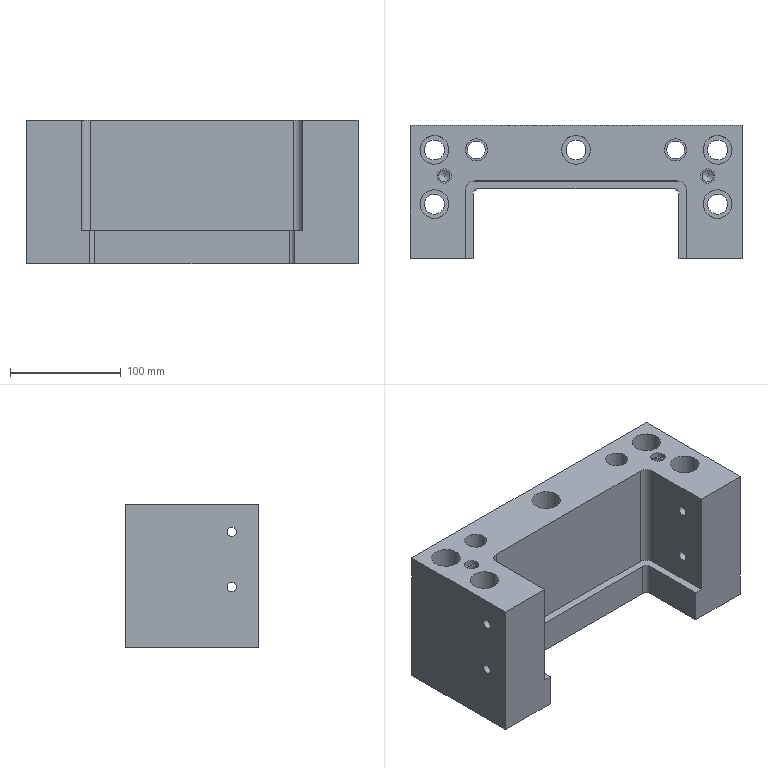Part | NX | features FD 2 | 1 solid | 51 faces | box 300 x 120 x 130 mm | volume 2560198 mm3 | cylinder 26 | plane 23 | cone 2 | commonest cylinder face diameters 18 x5 26 x5 8.5 x4 10 x2 10.3 x2 13 x2
STEP:
#1=CARTESIAN_POINT('',(1053.,-648.5,-33.75));
#2=VERTEX_POINT('',#1);
#3=CARTESIAN_POINT('',(1053.,-648.5,-38.));
#4=DIRECTION('',(-1.,0.,0.));
#5=DIRECTION('',(0.,0.,1.));
#6=AXIS2_PLACEMENT_3D('',#3,#4,#5);
#7=CIRCLE('',#6,4.25);
#8=EDGE_CURVE('',#2,#2,#7,.T.);
#9=ORIENTED_EDGE('',*,*,#8,.T.);
#10=EDGE_LOOP('',(#9));
#11=FACE_BOUND('',#10,.T.);
#12=CARTESIAN_POINT('',(1053.,-648.5,-83.75));
#13=VERTEX_POINT('',#12);
#14=CARTESIAN_POINT('',(1053.,-648.5,-88.));
#15=DIRECTION('',(-1.,0.,0.));
#16=DIRECTION('',(0.,0.,1.));
#17=AXIS2_PLACEMENT_3D('',#14,#15,#16);
#18=CIRCLE('',#17,4.25);
#19=EDGE_CURVE('',#13,#13,#18,.T.);
#20=ORIENTED_EDGE('',*,*,#19,.T.);
#21=EDGE_LOOP('',(#20));
#22=FACE_BOUND('',#21,.T.);
#23=CARTESIAN_POINT('',(1053.,-672.5,-13.));
#24=VERTEX_POINT('',#23);
#25=CARTESIAN_POINT('',(1053.,-672.5,-143.));
#26=VERTEX_POINT('',#25);
#27=CARTESIAN_POINT('',(1053.,-672.5,-3.));
#28=DIRECTION('',(0.,0.,-1.));
#29=VECTOR('',#28,1000.);
#30=LINE('',#27,#29);
#31=EDGE_CURVE('',#24,#26,#30,.T.);
#32=ORIENTED_EDGE('',*,*,#31,.T.);
#33=CARTESIAN_POINT('',(1053.,-552.5,-143.));
#34=VERTEX_POINT('',#33);
#35=CARTESIAN_POINT('',(1053.,-639.99,-143.));
#36=DIRECTION('',(0.,-1.,0.));
#37=VECTOR('',#36,1000.);
#38=LINE('',#35,#37);
#39=EDGE_CURVE('',#34,#26,#38,.T.);
#40=ORIENTED_EDGE('',*,*,#39,.F.);
#41=CARTESIAN_POINT('',(1053.,-552.5,-13.));
#42=VERTEX_POINT('',#41);
#43=CARTESIAN_POINT('',(1053.,-552.5,-3.));
#44=DIRECTION('',(0.,0.,-1.));
#45=VECTOR('',#44,1000.);
#46=LINE('',#43,#45);
#47=EDGE_CURVE('',#42,#34,#46,.T.);
#48=ORIENTED_EDGE('',*,*,#47,.F.);
#49=CARTESIAN_POINT('',(1053.,-667.5,-13.));
#50=DIRECTION('',(0.,-1.,0.));
#51=VECTOR('',#50,1000.);
#52=LINE('',#49,#51);
#53=EDGE_CURVE('',#42,#24,#52,.T.);
#54=ORIENTED_EDGE('',*,*,#53,.T.);
#55=EDGE_LOOP('',(#32,#40,#48,#54));
#56=FACE_BOUND('',#55,.T.);
#57=CARTESIAN_POINT('',(1053.,-667.5,202.));
#58=DIRECTION('',(-1.,0.,0.));
#59=DIRECTION('',(0.,0.,-1.));
#60=AXIS2_PLACEMENT_3D('',#57,#58,#59);
#61=PLANE('',#60);
#62=ADVANCED_FACE('',(#11,#22,#56),#61,.F.);
#63=CARTESIAN_POINT('',(803.,-648.5,-42.25));
#64=VERTEX_POINT('',#63);
#65=CARTESIAN_POINT('',(803.,-648.5,-38.));
#66=DIRECTION('',(1.,0.,0.));
#67=DIRECTION('',(0.,0.,-1.));
#68=AXIS2_PLACEMENT_3D('',#65,#66,#67);
#69=CIRCLE('',#68,4.25);
#70=EDGE_CURVE('',#64,#64,#69,.T.);
#71=ORIENTED_EDGE('',*,*,#70,.F.);
#72=EDGE_LOOP('',(#71));
#73=FACE_BOUND('',#72,.T.);
#74=CARTESIAN_POINT('',(803.,-648.5,-92.25));
#75=VERTEX_POINT('',#74);
#76=CARTESIAN_POINT('',(803.,-648.5,-88.));
#77=DIRECTION('',(1.,0.,0.));
#78=DIRECTION('',(0.,0.,-1.));
#79=AXIS2_PLACEMENT_3D('',#76,#77,#78);
#80=CIRCLE('',#79,4.25);
#81=EDGE_CURVE('',#75,#75,#80,.T.);
#82=ORIENTED_EDGE('',*,*,#81,.F.);
#83=EDGE_LOOP('',(#82));
#84=FACE_BOUND('',#83,.T.);
#85=CARTESIAN_POINT('',(803.,-672.5,-113.));
#86=VERTEX_POINT('',#85);
#87=CARTESIAN_POINT('',(803.,-610.5,-113.));
#88=VERTEX_POINT('',#87);
#89=CARTESIAN_POINT('',(803.,-674.98,-113.));
#90=DIRECTION('',(0.,1.,0.));
#91=VECTOR('',#90,1000.);
#92=LINE('',#89,#91);
#93=EDGE_CURVE('',#86,#88,#92,.T.);
#94=ORIENTED_EDGE('',*,*,#93,.T.);
#95=CARTESIAN_POINT('',(803.,-610.5,-13.));
#96=VERTEX_POINT('',#95);
#97=CARTESIAN_POINT('',(803.,-610.5,-113.));
#98=DIRECTION('',(0.,0.,-1.));
#99=VECTOR('',#98,1000.);
#100=LINE('',#97,#99);
#101=EDGE_CURVE('',#96,#88,#100,.T.);
#102=ORIENTED_EDGE('',*,*,#101,.F.);
#103=CARTESIAN_POINT('',(803.,-672.5,-13.));
#104=VERTEX_POINT('',#103);
#105=CARTESIAN_POINT('',(803.,-674.98,-13.));
#106=DIRECTION('',(0.,1.,0.));
#107=VECTOR('',#106,1000.);
#108=LINE('',#105,#107);
#109=EDGE_CURVE('',#104,#96,#108,.T.);
#110=ORIENTED_EDGE('',*,*,#109,.F.);
#111=CARTESIAN_POINT('',(803.,-672.5,-3.));
#112=DIRECTION('',(0.,0.,1.));
#113=VECTOR('',#112,1000.);
#114=LINE('',#111,#113);
#115=EDGE_CURVE('',#86,#104,#114,.T.);
#116=ORIENTED_EDGE('',*,*,#115,.F.);
#117=EDGE_LOOP('',(#94,#102,#110,#116));
#118=FACE_BOUND('',#117,.T.);
#119=CARTESIAN_POINT('',(803.,-674.98,-113.));
#120=DIRECTION('',(-1.,0.,0.));
#121=DIRECTION('',(0.,0.,1.));
#122=AXIS2_PLACEMENT_3D('',#119,#120,#121);
#123=PLANE('',#122);
#124=ADVANCED_FACE('',(#73,#84,#118),#123,.F.);
#125=CARTESIAN_POINT('',(811.,-602.5,-113.));
#126=VERTEX_POINT('',#125);
#127=CARTESIAN_POINT('',(811.,-610.5,-113.));
#128=DIRECTION('',(0.,0.,-1.));
#129=DIRECTION('',(-1.,0.,0.));
#130=AXIS2_PLACEMENT_3D('',#127,#128,#129);
#131=CIRCLE('',#130,8.);
#132=EDGE_CURVE('',#88,#126,#131,.T.);
#133=ORIENTED_EDGE('',*,*,#132,.T.);
#134=CARTESIAN_POINT('',(811.,-602.5,-13.));
#135=VERTEX_POINT('',#134);
#136=CARTESIAN_POINT('',(811.,-602.5,-13.));
#137=DIRECTION('',(0.,0.,1.));
#138=VECTOR('',#137,1000.);
#139=LINE('',#136,#138);
#140=EDGE_CURVE('',#126,#135,#139,.T.);
#141=ORIENTED_EDGE('',*,*,#140,.T.);
#142=CARTESIAN_POINT('',(811.,-610.5,-13.));
#143=DIRECTION('',(0.,0.,1.));
#144=DIRECTION('',(-1.,0.,0.));
#145=AXIS2_PLACEMENT_3D('',#142,#143,#144);
#146=CIRCLE('',#145,8.);
#147=EDGE_CURVE('',#135,#96,#146,.T.);
#148=ORIENTED_EDGE('',*,*,#147,.T.);
#149=ORIENTED_EDGE('',*,*,#101,.T.);
#150=EDGE_LOOP('',(#133,#141,#148,#149));
#151=FACE_BOUND('',#150,.T.);
#152=CARTESIAN_POINT('',(811.,-610.5,-113.));
#153=DIRECTION('',(0.,0.,1.));
#154=DIRECTION('',(-1.,0.,0.));
#155=AXIS2_PLACEMENT_3D('',#152,#153,#154);
#156=CYLINDRICAL_SURFACE('',#155,8.);
#157=ADVANCED_FACE('',(#151),#156,.F.);
#158=CARTESIAN_POINT('',(995.,-602.5,-113.));
#159=VERTEX_POINT('',#158);
#160=CARTESIAN_POINT('',(832.96,-602.5,-113.));
#161=DIRECTION('',(-1.,0.,0.));
#162=VECTOR('',#161,1000.);
#163=LINE('',#160,#162);
#164=EDGE_CURVE('',#159,#126,#163,.T.);
#165=ORIENTED_EDGE('',*,*,#164,.F.);
#166=CARTESIAN_POINT('',(995.,-602.5,-13.));
#167=VERTEX_POINT('',#166);
#168=CARTESIAN_POINT('',(995.,-602.5,-113.));
#169=DIRECTION('',(0.,0.,-1.));
#170=VECTOR('',#169,1000.);
#171=LINE('',#168,#170);
#172=EDGE_CURVE('',#167,#159,#171,.T.);
#173=ORIENTED_EDGE('',*,*,#172,.F.);
#174=CARTESIAN_POINT('',(832.96,-602.5,-13.));
#175=DIRECTION('',(1.,0.,0.));
#176=VECTOR('',#175,1000.);
#177=LINE('',#174,#176);
#178=EDGE_CURVE('',#135,#167,#177,.T.);
#179=ORIENTED_EDGE('',*,*,#178,.F.);
#180=ORIENTED_EDGE('',*,*,#140,.F.);
#181=EDGE_LOOP('',(#165,#173,#179,#180));
#182=FACE_BOUND('',#181,.T.);
#183=CARTESIAN_POINT('',(832.96,-602.5,-113.));
#184=DIRECTION('',(0.,1.,0.));
#185=DIRECTION('',(0.,0.,-1.));
#186=AXIS2_PLACEMENT_3D('',#183,#184,#185);
#187=PLANE('',#186);
#188=ADVANCED_FACE('',(#182),#187,.F.);
#189=CARTESIAN_POINT('',(1003.,-610.5,-113.));
#190=VERTEX_POINT('',#189);
#191=CARTESIAN_POINT('',(995.,-610.5,-113.));
#192=DIRECTION('',(0.,0.,1.));
#193=DIRECTION('',(-1.,0.,0.));
#194=AXIS2_PLACEMENT_3D('',#191,#192,#193);
#195=CIRCLE('',#194,8.);
#196=EDGE_CURVE('',#190,#159,#195,.T.);
#197=ORIENTED_EDGE('',*,*,#196,.F.);
#198=CARTESIAN_POINT('',(1003.,-610.5,-13.));
#199=VERTEX_POINT('',#198);
#200=CARTESIAN_POINT('',(1003.,-610.5,-113.));
#201=DIRECTION('',(0.,0.,1.));
#202=VECTOR('',#201,1000.);
#203=LINE('',#200,#202);
#204=EDGE_CURVE('',#190,#199,#203,.T.);
#205=ORIENTED_EDGE('',*,*,#204,.T.);
#206=CARTESIAN_POINT('',(995.,-610.5,-13.));
#207=DIRECTION('',(0.,0.,1.));
#208=DIRECTION('',(-1.,0.,0.));
#209=AXIS2_PLACEMENT_3D('',#206,#207,#208);
#210=CIRCLE('',#209,8.);
#211=EDGE_CURVE('',#199,#167,#210,.T.);
#212=ORIENTED_EDGE('',*,*,#211,.T.);
#213=ORIENTED_EDGE('',*,*,#172,.T.);
#214=EDGE_LOOP('',(#197,#205,#212,#213));
#215=FACE_BOUND('',#214,.T.);
#216=CARTESIAN_POINT('',(995.,-610.5,-113.));
#217=DIRECTION('',(0.,0.,1.));
#218=DIRECTION('',(-1.,0.,0.));
#219=AXIS2_PLACEMENT_3D('',#216,#217,#218);
#220=CYLINDRICAL_SURFACE('',#219,8.);
#221=ADVANCED_FACE('',(#215),#220,.F.);
#222=CARTESIAN_POINT('',(1003.,-648.5,-33.75));
#223=VERTEX_POINT('',#222);
#224=CARTESIAN_POINT('',(1003.,-648.5,-38.));
#225=DIRECTION('',(-1.,0.,0.));
#226=DIRECTION('',(0.,0.,1.));
#227=AXIS2_PLACEMENT_3D('',#224,#225,#226);
#228=CIRCLE('',#227,4.25);
#229=EDGE_CURVE('',#223,#223,#228,.T.);
#230=ORIENTED_EDGE('',*,*,#229,.F.);
#231=EDGE_LOOP('',(#230));
#232=FACE_BOUND('',#231,.T.);
#233=CARTESIAN_POINT('',(1003.,-648.5,-83.75));
#234=VERTEX_POINT('',#233);
#235=CARTESIAN_POINT('',(1003.,-648.5,-88.));
#236=DIRECTION('',(-1.,0.,0.));
#237=DIRECTION('',(0.,0.,1.));
#238=AXIS2_PLACEMENT_3D('',#235,#236,#237);
#239=CIRCLE('',#238,4.25);
#240=EDGE_CURVE('',#234,#234,#239,.T.);
#241=ORIENTED_EDGE('',*,*,#240,.F.);
#242=EDGE_LOOP('',(#241));
#243=FACE_BOUND('',#242,.T.);
#244=CARTESIAN_POINT('',(1003.,-672.5,-113.));
#245=VERTEX_POINT('',#244);
#246=CARTESIAN_POINT('',(1003.,-612.48,-113.));
#247=DIRECTION('',(0.,1.,0.));
#248=VECTOR('',#247,1000.);
#249=LINE('',#246,#248);
#250=EDGE_CURVE('',#245,#190,#249,.T.);
#251=ORIENTED_EDGE('',*,*,#250,.F.);
#252=CARTESIAN_POINT('',(1003.,-672.5,-13.));
#253=VERTEX_POINT('',#252);
#254=CARTESIAN_POINT('',(1003.,-672.5,-3.));
#255=DIRECTION('',(0.,0.,-1.));
#256=VECTOR('',#255,1000.);
#257=LINE('',#254,#256);
#258=EDGE_CURVE('',#253,#245,#257,.T.);
#259=ORIENTED_EDGE('',*,*,#258,.F.);
#260=CARTESIAN_POINT('',(1003.,-612.48,-13.));
#261=DIRECTION('',(0.,-1.,0.));
#262=VECTOR('',#261,1000.);
#263=LINE('',#260,#262);
#264=EDGE_CURVE('',#199,#253,#263,.T.);
#265=ORIENTED_EDGE('',*,*,#264,.F.);
#266=ORIENTED_EDGE('',*,*,#204,.F.);
#267=EDGE_LOOP('',(#251,#259,#265,#266));
#268=FACE_BOUND('',#267,.T.);
#269=CARTESIAN_POINT('',(1003.,-612.48,-113.));
#270=DIRECTION('',(1.,0.,0.));
#271=DIRECTION('',(0.,0.,-1.));
#272=AXIS2_PLACEMENT_3D('',#269,#270,#271);
#273=PLANE('',#272);
#274=ADVANCED_FACE('',(#232,#243,#268),#273,.F.);
#275=ORIENTED_EDGE('',*,*,#258,.T.);
#276=CARTESIAN_POINT('',(996.,-672.5,-113.));
#277=VERTEX_POINT('',#276);
#278=CARTESIAN_POINT('',(1007.98,-672.5,-113.));
#279=DIRECTION('',(1.,0.,0.));
#280=VECTOR('',#279,1000.);
#281=LINE('',#278,#280);
#282=EDGE_CURVE('',#277,#245,#281,.T.);
#283=ORIENTED_EDGE('',*,*,#282,.F.);
#284=CARTESIAN_POINT('',(996.,-672.5,-143.));
#285=VERTEX_POINT('',#284);
#286=CARTESIAN_POINT('',(996.,-672.5,-113.));
#287=DIRECTION('',(0.,0.,-1.));
#288=VECTOR('',#287,1000.);
#289=LINE('',#286,#288);
#290=EDGE_CURVE('',#277,#285,#289,.T.);
#291=ORIENTED_EDGE('',*,*,#290,.T.);
#292=CARTESIAN_POINT('',(1007.98,-672.5,-143.));
#293=DIRECTION('',(-1.,0.,0.));
#294=VECTOR('',#293,1000.);
#295=LINE('',#292,#294);
#296=EDGE_CURVE('',#26,#285,#295,.T.);
#297=ORIENTED_EDGE('',*,*,#296,.F.);
#298=ORIENTED_EDGE('',*,*,#31,.F.);
#299=CARTESIAN_POINT('',(1007.98,-672.5,-13.));
#300=DIRECTION('',(1.,0.,0.));
#301=VECTOR('',#300,1000.);
#302=LINE('',#299,#301);
#303=EDGE_CURVE('',#253,#24,#302,.T.);
#304=ORIENTED_EDGE('',*,*,#303,.F.);
#305=EDGE_LOOP('',(#275,#283,#291,#297,#298,#304));
#306=FACE_BOUND('',#305,.T.);
#307=CARTESIAN_POINT('',(1007.98,-672.5,-3.));
#308=DIRECTION('',(0.,-1.,0.));
#309=DIRECTION('',(0.,0.,1.));
#310=AXIS2_PLACEMENT_3D('',#307,#308,#309);
#311=PLANE('',#310);
#312=ADVANCED_FACE('',(#306),#311,.T.);
#313=CARTESIAN_POINT('',(753.,-672.5,-13.));
#314=VERTEX_POINT('',#313);
#315=CARTESIAN_POINT('',(753.,-672.5,-143.));
#316=VERTEX_POINT('',#315);
#317=CARTESIAN_POINT('',(753.,-672.5,202.));
#318=DIRECTION('',(0.,0.,-1.));
#319=VECTOR('',#318,1000.);
#320=LINE('',#317,#319);
#321=EDGE_CURVE('',#314,#316,#320,.T.);
#322=ORIENTED_EDGE('',*,*,#321,.T.);
#323=CARTESIAN_POINT('',(810.,-672.5,-143.));
#324=VERTEX_POINT('',#323);
#325=CARTESIAN_POINT('',(797.98,-672.5,-143.));
#326=DIRECTION('',(-1.,0.,0.));
#327=VECTOR('',#326,1000.);
#328=LINE('',#325,#327);
#329=EDGE_CURVE('',#324,#316,#328,.T.);
#330=ORIENTED_EDGE('',*,*,#329,.F.);
#331=CARTESIAN_POINT('',(810.,-672.5,-113.));
#332=VERTEX_POINT('',#331);
#333=CARTESIAN_POINT('',(810.,-672.5,-3.));
#334=DIRECTION('',(0.,0.,1.));
#335=VECTOR('',#334,1000.);
#336=LINE('',#333,#335);
#337=EDGE_CURVE('',#324,#332,#336,.T.);
#338=ORIENTED_EDGE('',*,*,#337,.T.);
#339=CARTESIAN_POINT('',(797.98,-672.5,-113.));
#340=DIRECTION('',(1.,0.,0.));
#341=VECTOR('',#340,1000.);
#342=LINE('',#339,#341);
#343=EDGE_CURVE('',#86,#332,#342,.T.);
#344=ORIENTED_EDGE('',*,*,#343,.F.);
#345=ORIENTED_EDGE('',*,*,#115,.T.);
#346=CARTESIAN_POINT('',(797.98,-672.5,-13.));
#347=DIRECTION('',(-1.,0.,0.));
#348=VECTOR('',#347,1000.);
#349=LINE('',#346,#348);
#350=EDGE_CURVE('',#104,#314,#349,.T.);
#351=ORIENTED_EDGE('',*,*,#350,.T.);
#352=EDGE_LOOP('',(#322,#330,#338,#344,#345,#351));
#353=FACE_BOUND('',#352,.T.);
#354=CARTESIAN_POINT('',(797.98,-672.5,-3.));
#355=DIRECTION('',(0.,1.,0.));
#356=DIRECTION('',(0.,0.,1.));
#357=AXIS2_PLACEMENT_3D('',#354,#355,#356);
#358=PLANE('',#357);
#359=ADVANCED_FACE('',(#353),#358,.F.);
#360=CARTESIAN_POINT('',(753.,-648.5,-42.25));
#361=VERTEX_POINT('',#360);
#362=CARTESIAN_POINT('',(753.,-648.5,-38.));
#363=DIRECTION('',(1.,0.,0.));
#364=DIRECTION('',(0.,0.,-1.));
#365=AXIS2_PLACEMENT_3D('',#362,#363,#364);
#366=CIRCLE('',#365,4.25);
#367=EDGE_CURVE('',#361,#361,#366,.T.);
#368=ORIENTED_EDGE('',*,*,#367,.T.);
#369=EDGE_LOOP('',(#368));
#370=FACE_BOUND('',#369,.T.);
#371=CARTESIAN_POINT('',(753.,-648.5,-92.25));
#372=VERTEX_POINT('',#371);
#373=CARTESIAN_POINT('',(753.,-648.5,-88.));
#374=DIRECTION('',(1.,0.,0.));
#375=DIRECTION('',(0.,0.,-1.));
#376=AXIS2_PLACEMENT_3D('',#373,#374,#375);
#377=CIRCLE('',#376,4.25);
#378=EDGE_CURVE('',#372,#372,#377,.T.);
#379=ORIENTED_EDGE('',*,*,#378,.T.);
#380=EDGE_LOOP('',(#379));
#381=FACE_BOUND('',#380,.T.);
#382=CARTESIAN_POINT('',(753.,-552.5,-13.));
#383=VERTEX_POINT('',#382);
#384=CARTESIAN_POINT('',(753.,-552.5,-143.));
#385=VERTEX_POINT('',#384);
#386=CARTESIAN_POINT('',(753.,-552.5,202.));
#387=DIRECTION('',(0.,0.,-1.));
#388=VECTOR('',#387,1000.);
#389=LINE('',#386,#388);
#390=EDGE_CURVE('',#383,#385,#389,.T.);
#391=ORIENTED_EDGE('',*,*,#390,.T.);
#392=CARTESIAN_POINT('',(753.,-639.99,-143.));
#393=DIRECTION('',(0.,1.,0.));
#394=VECTOR('',#393,1000.);
#395=LINE('',#392,#394);
#396=EDGE_CURVE('',#316,#385,#395,.T.);
#397=ORIENTED_EDGE('',*,*,#396,.F.);
#398=ORIENTED_EDGE('',*,*,#321,.F.);
#399=CARTESIAN_POINT('',(753.,-667.5,-13.));
#400=DIRECTION('',(0.,1.,0.));
#401=VECTOR('',#400,1000.);
#402=LINE('',#399,#401);
#403=EDGE_CURVE('',#314,#383,#402,.T.);
#404=ORIENTED_EDGE('',*,*,#403,.T.);
#405=EDGE_LOOP('',(#391,#397,#398,#404));
#406=FACE_BOUND('',#405,.T.);
#407=CARTESIAN_POINT('',(753.,-622.5,202.));
#408=DIRECTION('',(1.,0.,0.));
#409=DIRECTION('',(0.,0.,1.));
#410=AXIS2_PLACEMENT_3D('',#407,#408,#409);
#411=PLANE('',#410);
#412=ADVANCED_FACE('',(#370,#381,#406),#411,.F.);
#413=ORIENTED_EDGE('',*,*,#47,.T.);
#414=CARTESIAN_POINT('',(827.98,-552.5,-143.));
#415=DIRECTION('',(1.,0.,0.));
#416=VECTOR('',#415,1000.);
#417=LINE('',#414,#416);
#418=EDGE_CURVE('',#385,#34,#417,.T.);
#419=ORIENTED_EDGE('',*,*,#418,.F.);
#420=ORIENTED_EDGE('',*,*,#390,.F.);
#421=CARTESIAN_POINT('',(827.98,-552.5,-13.));
#422=DIRECTION('',(1.,0.,0.));
#423=VECTOR('',#422,1000.);
#424=LINE('',#421,#423);
#425=EDGE_CURVE('',#383,#42,#424,.T.);
#426=ORIENTED_EDGE('',*,*,#425,.T.);
#427=EDGE_LOOP('',(#413,#419,#420,#426));
#428=FACE_BOUND('',#427,.T.);
#429=CARTESIAN_POINT('',(827.98,-552.5,-3.));
#430=DIRECTION('',(0.,-1.,0.));
#431=DIRECTION('',(0.,0.,1.));
#432=AXIS2_PLACEMENT_3D('',#429,#430,#431);
#433=PLANE('',#432);
#434=ADVANCED_FACE('',(#428),#433,.F.);
#435=CARTESIAN_POINT('',(985.,-574.5,-67.));
#436=VERTEX_POINT('',#435);
#437=CARTESIAN_POINT('',(993.,-574.5,-67.));
#438=DIRECTION('',(0.,0.,-1.));
#439=DIRECTION('',(-1.,0.,0.));
#440=AXIS2_PLACEMENT_3D('',#437,#438,#439);
#441=CIRCLE('',#440,8.001);
#442=EDGE_CURVE('',#436,#436,#441,.T.);
#443=ORIENTED_EDGE('',*,*,#442,.F.);
#444=EDGE_LOOP('',(#443));
#445=FACE_BOUND('',#444,.T.);
#446=CARTESIAN_POINT('',(1001.,-574.5,-143.));
#447=VERTEX_POINT('',#446);
#448=CARTESIAN_POINT('',(993.,-574.5,-143.));
#449=DIRECTION('',(0.,0.,1.));
#450=DIRECTION('',(1.,0.,0.));
#451=AXIS2_PLACEMENT_3D('',#448,#449,#450);
#452=CIRCLE('',#451,8.001);
#453=EDGE_CURVE('',#447,#447,#452,.T.);
#454=ORIENTED_EDGE('',*,*,#453,.F.);
#455=EDGE_LOOP('',(#454));
#456=FACE_BOUND('',#455,.T.);
#457=CARTESIAN_POINT('',(993.,-574.5,-11.));
#458=DIRECTION('',(0.,0.,-1.));
#459=DIRECTION('',(1.,0.,0.));
#460=AXIS2_PLACEMENT_3D('',#457,#458,#459);
#461=CYLINDRICAL_SURFACE('',#460,8.001);
#462=ADVANCED_FACE('',(#445,#456),#461,.F.);
#463=CARTESIAN_POINT('',(1022.,-623.5,-103.));
#464=VERTEX_POINT('',#463);
#465=CARTESIAN_POINT('',(1031.,-623.5,-103.));
#466=DIRECTION('',(0.,0.,-1.));
#467=DIRECTION('',(-1.,0.,0.));
#468=AXIS2_PLACEMENT_3D('',#465,#466,#467);
#469=CIRCLE('',#468,9.);
#470=EDGE_CURVE('',#464,#464,#469,.T.);
#471=ORIENTED_EDGE('',*,*,#470,.F.);
#472=EDGE_LOOP('',(#471));
#473=FACE_BOUND('',#472,.T.);
#474=CARTESIAN_POINT('',(1040.,-623.5,-143.));
#475=VERTEX_POINT('',#474);
#476=CARTESIAN_POINT('',(1031.,-623.5,-143.));
#477=DIRECTION('',(0.,0.,1.));
#478=DIRECTION('',(1.,0.,0.));
#479=AXIS2_PLACEMENT_3D('',#476,#477,#478);
#480=CIRCLE('',#479,9.);
#481=EDGE_CURVE('',#475,#475,#480,.T.);
#482=ORIENTED_EDGE('',*,*,#481,.F.);
#483=EDGE_LOOP('',(#482));
#484=FACE_BOUND('',#483,.T.);
#485=CARTESIAN_POINT('',(1031.,-623.5,-11.));
#486=DIRECTION('',(0.,0.,-1.));
#487=DIRECTION('',(-1.,0.,0.));
#488=AXIS2_PLACEMENT_3D('',#485,#486,#487);
#489=CYLINDRICAL_SURFACE('',#488,9.);
#490=ADVANCED_FACE('',(#473,#484),#489,.F.);
#491=CARTESIAN_POINT('',(766.,-574.5,-103.));
#492=VERTEX_POINT('',#491);
#493=CARTESIAN_POINT('',(775.,-574.5,-103.));
#494=DIRECTION('',(0.,0.,-1.));
#495=DIRECTION('',(-1.,0.,0.));
#496=AXIS2_PLACEMENT_3D('',#493,#494,#495);
#497=CIRCLE('',#496,9.);
#498=EDGE_CURVE('',#492,#492,#497,.T.);
#499=ORIENTED_EDGE('',*,*,#498,.F.);
#500=EDGE_LOOP('',(#499));
#501=FACE_BOUND('',#500,.T.);
#502=CARTESIAN_POINT('',(784.,-574.5,-143.));
#503=VERTEX_POINT('',#502);
#504=CARTESIAN_POINT('',(775.,-574.5,-143.));
#505=DIRECTION('',(0.,0.,1.));
#506=DIRECTION('',(1.,0.,0.));
#507=AXIS2_PLACEMENT_3D('',#504,#505,#506);
#508=CIRCLE('',#507,9.);
#509=EDGE_CURVE('',#503,#503,#508,.T.);
#510=ORIENTED_EDGE('',*,*,#509,.F.);
#511=EDGE_LOOP('',(#510));
#512=FACE_BOUND('',#511,.T.);
#513=CARTESIAN_POINT('',(775.,-574.5,-11.));
#514=DIRECTION('',(0.,0.,-1.));
#515=DIRECTION('',(-1.,0.,0.));
#516=AXIS2_PLACEMENT_3D('',#513,#514,#515);
#517=CYLINDRICAL_SURFACE('',#516,9.);
#518=ADVANCED_FACE('',(#501,#512),#517,.F.);
#519=CARTESIAN_POINT('',(894.,-574.5,-103.));
#520=VERTEX_POINT('',#519);
#521=CARTESIAN_POINT('',(903.,-574.5,-103.));
#522=DIRECTION('',(0.,0.,-1.));
#523=DIRECTION('',(-1.,0.,0.));
#524=AXIS2_PLACEMENT_3D('',#521,#522,#523);
#525=CIRCLE('',#524,9.);
#526=EDGE_CURVE('',#520,#520,#525,.T.);
#527=ORIENTED_EDGE('',*,*,#526,.F.);
#528=EDGE_LOOP('',(#527));
#529=FACE_BOUND('',#528,.T.);
#530=CARTESIAN_POINT('',(912.,-574.5,-143.));
#531=VERTEX_POINT('',#530);
#532=CARTESIAN_POINT('',(903.,-574.5,-143.));
#533=DIRECTION('',(0.,0.,1.));
#534=DIRECTION('',(1.,0.,0.));
#535=AXIS2_PLACEMENT_3D('',#532,#533,#534);
#536=CIRCLE('',#535,9.);
#537=EDGE_CURVE('',#531,#531,#536,.T.);
#538=ORIENTED_EDGE('',*,*,#537,.F.);
#539=EDGE_LOOP('',(#538));
#540=FACE_BOUND('',#539,.T.);
#541=CARTESIAN_POINT('',(903.,-574.5,-11.));
#542=DIRECTION('',(0.,0.,-1.));
#543=DIRECTION('',(-1.,0.,0.));
#544=AXIS2_PLACEMENT_3D('',#541,#542,#543);
#545=CYLINDRICAL_SURFACE('',#544,9.);
#546=ADVANCED_FACE('',(#529,#540),#545,.F.);
#547=CARTESIAN_POINT('',(1022.,-574.5,-103.));
#548=VERTEX_POINT('',#547);
#549=CARTESIAN_POINT('',(1031.,-574.5,-103.));
#550=DIRECTION('',(0.,0.,-1.));
#551=DIRECTION('',(-1.,0.,0.));
#552=AXIS2_PLACEMENT_3D('',#549,#550,#551);
#553=CIRCLE('',#552,9.);
#554=EDGE_CURVE('',#548,#548,#553,.T.);
#555=ORIENTED_EDGE('',*,*,#554,.F.);
#556=EDGE_LOOP('',(#555));
#557=FACE_BOUND('',#556,.T.);
#558=CARTESIAN_POINT('',(1040.,-574.5,-143.));
#559=VERTEX_POINT('',#558);
#560=CARTESIAN_POINT('',(1031.,-574.5,-143.));
#561=DIRECTION('',(0.,0.,1.));
#562=DIRECTION('',(1.,0.,0.));
#563=AXIS2_PLACEMENT_3D('',#560,#561,#562);
#564=CIRCLE('',#563,9.);
#565=EDGE_CURVE('',#559,#559,#564,.T.);
#566=ORIENTED_EDGE('',*,*,#565,.F.);
#567=EDGE_LOOP('',(#566));
#568=FACE_BOUND('',#567,.T.);
#569=CARTESIAN_POINT('',(1031.,-574.5,-11.));
#570=DIRECTION('',(0.,0.,-1.));
#571=DIRECTION('',(-1.,0.,0.));
#572=AXIS2_PLACEMENT_3D('',#569,#570,#571);
#573=CYLINDRICAL_SURFACE('',#572,9.);
#574=ADVANCED_FACE('',(#557,#568),#573,.F.);
#575=CARTESIAN_POINT('',(805.,-574.5,-67.));
#576=VERTEX_POINT('',#575);
#577=CARTESIAN_POINT('',(813.,-574.5,-67.));
#578=DIRECTION('',(0.,0.,-1.));
#579=DIRECTION('',(-1.,0.,0.));
#580=AXIS2_PLACEMENT_3D('',#577,#578,#579);
#581=CIRCLE('',#580,8.001);
#582=EDGE_CURVE('',#576,#576,#581,.T.);
#583=ORIENTED_EDGE('',*,*,#582,.F.);
#584=EDGE_LOOP('',(#583));
#585=FACE_BOUND('',#584,.T.);
#586=CARTESIAN_POINT('',(821.,-574.5,-143.));
#587=VERTEX_POINT('',#586);
#588=CARTESIAN_POINT('',(813.,-574.5,-143.));
#589=DIRECTION('',(0.,0.,1.));
#590=DIRECTION('',(1.,0.,0.));
#591=AXIS2_PLACEMENT_3D('',#588,#589,#590);
#592=CIRCLE('',#591,8.001);
#593=EDGE_CURVE('',#587,#587,#592,.T.);
#594=ORIENTED_EDGE('',*,*,#593,.F.);
#595=EDGE_LOOP('',(#594));
#596=FACE_BOUND('',#595,.T.);
#597=CARTESIAN_POINT('',(813.,-574.5,-11.));
#598=DIRECTION('',(0.,0.,-1.));
#599=DIRECTION('',(-1.,0.,0.));
#600=AXIS2_PLACEMENT_3D('',#597,#598,#599);
#601=CYLINDRICAL_SURFACE('',#600,8.001);
#602=ADVANCED_FACE('',(#585,#596),#601,.F.);
#603=CARTESIAN_POINT('',(766.,-623.5,-103.));
#604=VERTEX_POINT('',#603);
#605=CARTESIAN_POINT('',(775.,-623.5,-103.));
#606=DIRECTION('',(0.,0.,-1.));
#607=DIRECTION('',(-1.,0.,0.));
#608=AXIS2_PLACEMENT_3D('',#605,#606,#607);
#609=CIRCLE('',#608,9.);
#610=EDGE_CURVE('',#604,#604,#609,.T.);
#611=ORIENTED_EDGE('',*,*,#610,.F.);
#612=EDGE_LOOP('',(#611));
#613=FACE_BOUND('',#612,.T.);
#614=CARTESIAN_POINT('',(784.,-623.5,-143.));
#615=VERTEX_POINT('',#614);
#616=CARTESIAN_POINT('',(775.,-623.5,-143.));
#617=DIRECTION('',(0.,0.,1.));
#618=DIRECTION('',(1.,0.,0.));
#619=AXIS2_PLACEMENT_3D('',#616,#617,#618);
#620=CIRCLE('',#619,9.);
#621=EDGE_CURVE('',#615,#615,#620,.T.);
#622=ORIENTED_EDGE('',*,*,#621,.F.);
#623=EDGE_LOOP('',(#622));
#624=FACE_BOUND('',#623,.T.);
#625=CARTESIAN_POINT('',(775.,-623.5,-11.));
#626=DIRECTION('',(0.,0.,-1.));
#627=DIRECTION('',(-1.,0.,0.));
#628=AXIS2_PLACEMENT_3D('',#625,#626,#627);
#629=CYLINDRICAL_SURFACE('',#628,9.);
#630=ADVANCED_FACE('',(#613,#624),#629,.F.);
#631=CARTESIAN_POINT('',(1028.595,-598.139,-13.));
#632=VERTEX_POINT('',#631);
#633=CARTESIAN_POINT('',(1022.095,-598.139,-13.));
#634=DIRECTION('',(0.,0.,1.));
#635=DIRECTION('',(1.,0.,0.));
#636=AXIS2_PLACEMENT_3D('',#633,#634,#635);
#637=CIRCLE('',#636,6.5);
#638=EDGE_CURVE('',#632,#632,#637,.T.);
#639=ORIENTED_EDGE('',*,*,#638,.F.);
#640=EDGE_LOOP('',(#639));
#641=FACE_BOUND('',#640,.T.);
#642=CARTESIAN_POINT('',(777.405,-598.139,-13.));
#643=VERTEX_POINT('',#642);
#644=CARTESIAN_POINT('',(783.905,-598.139,-13.));
#645=DIRECTION('',(0.,0.,-1.));
#646=DIRECTION('',(-1.,0.,0.));
#647=AXIS2_PLACEMENT_3D('',#644,#645,#646);
#648=CIRCLE('',#647,6.5);
#649=EDGE_CURVE('',#643,#643,#648,.T.);
#650=ORIENTED_EDGE('',*,*,#649,.T.);
#651=EDGE_LOOP('',(#650));
#652=FACE_BOUND('',#651,.T.);
#653=CARTESIAN_POINT('',(1044.,-574.5,-13.));
#654=VERTEX_POINT('',#653);
#655=CARTESIAN_POINT('',(1031.,-574.5,-13.));
#656=DIRECTION('',(0.,0.,-1.));
#657=DIRECTION('',(1.,0.,0.));
#658=AXIS2_PLACEMENT_3D('',#655,#656,#657);
#659=CIRCLE('',#658,13.);
#660=EDGE_CURVE('',#654,#654,#659,.T.);
#661=ORIENTED_EDGE('',*,*,#660,.T.);
#662=EDGE_LOOP('',(#661));
#663=FACE_BOUND('',#662,.T.);
#664=CARTESIAN_POINT('',(788.,-574.5,-13.));
#665=VERTEX_POINT('',#664);
#666=CARTESIAN_POINT('',(775.,-574.5,-13.));
#667=DIRECTION('',(0.,0.,-1.));
#668=DIRECTION('',(1.,0.,0.));
#669=AXIS2_PLACEMENT_3D('',#666,#667,#668);
#670=CIRCLE('',#669,13.);
#671=EDGE_CURVE('',#665,#665,#670,.T.);
#672=ORIENTED_EDGE('',*,*,#671,.T.);
#673=EDGE_LOOP('',(#672));
#674=FACE_BOUND('',#673,.T.);
#675=ORIENTED_EDGE('',*,*,#403,.F.);
#676=ORIENTED_EDGE('',*,*,#350,.F.);
#677=ORIENTED_EDGE('',*,*,#109,.T.);
#678=ORIENTED_EDGE('',*,*,#147,.F.);
#679=ORIENTED_EDGE('',*,*,#178,.T.);
#680=ORIENTED_EDGE('',*,*,#211,.F.);
#681=ORIENTED_EDGE('',*,*,#264,.T.);
#682=ORIENTED_EDGE('',*,*,#303,.T.);
#683=ORIENTED_EDGE('',*,*,#53,.F.);
#684=ORIENTED_EDGE('',*,*,#425,.F.);
#685=EDGE_LOOP('',(#675,#676,#677,#678,#679,#680,#681,#682,#683,#684));
#686=FACE_BOUND('',#685,.T.);
#687=CARTESIAN_POINT('',(1003.,-574.5,-13.));
#688=VERTEX_POINT('',#687);
#689=CARTESIAN_POINT('',(993.,-574.5,-13.));
#690=DIRECTION('',(0.,0.,1.));
#691=DIRECTION('',(1.,0.,0.));
#692=AXIS2_PLACEMENT_3D('',#689,#690,#691);
#693=CIRCLE('',#692,10.);
#694=EDGE_CURVE('',#688,#688,#693,.T.);
#695=ORIENTED_EDGE('',*,*,#694,.F.);
#696=EDGE_LOOP('',(#695));
#697=FACE_BOUND('',#696,.T.);
#698=CARTESIAN_POINT('',(1044.,-623.5,-13.));
#699=VERTEX_POINT('',#698);
#700=CARTESIAN_POINT('',(1031.,-623.5,-13.));
#701=DIRECTION('',(0.,0.,-1.));
#702=DIRECTION('',(1.,0.,0.));
#703=AXIS2_PLACEMENT_3D('',#700,#701,#702);
#704=CIRCLE('',#703,13.);
#705=EDGE_CURVE('',#699,#699,#704,.T.);
#706=ORIENTED_EDGE('',*,*,#705,.T.);
#707=EDGE_LOOP('',(#706));
#708=FACE_BOUND('',#707,.T.);
#709=CARTESIAN_POINT('',(916.,-574.5,-13.));
#710=VERTEX_POINT('',#709);
#711=CARTESIAN_POINT('',(903.,-574.5,-13.));
#712=DIRECTION('',(0.,0.,-1.));
#713=DIRECTION('',(1.,0.,0.));
#714=AXIS2_PLACEMENT_3D('',#711,#712,#713);
#715=CIRCLE('',#714,13.);
#716=EDGE_CURVE('',#710,#710,#715,.T.);
#717=ORIENTED_EDGE('',*,*,#716,.T.);
#718=EDGE_LOOP('',(#717));
#719=FACE_BOUND('',#718,.T.);
#720=CARTESIAN_POINT('',(823.,-574.5,-13.));
#721=VERTEX_POINT('',#720);
#722=CARTESIAN_POINT('',(813.,-574.5,-13.));
#723=DIRECTION('',(0.,0.,1.));
#724=DIRECTION('',(1.,0.,0.));
#725=AXIS2_PLACEMENT_3D('',#722,#723,#724);
#726=CIRCLE('',#725,10.);
#727=EDGE_CURVE('',#721,#721,#726,.T.);
#728=ORIENTED_EDGE('',*,*,#727,.F.);
#729=EDGE_LOOP('',(#728));
#730=FACE_BOUND('',#729,.T.);
#731=CARTESIAN_POINT('',(788.,-623.5,-13.));
#732=VERTEX_POINT('',#731);
#733=CARTESIAN_POINT('',(775.,-623.5,-13.));
#734=DIRECTION('',(0.,0.,-1.));
#735=DIRECTION('',(1.,0.,0.));
#736=AXIS2_PLACEMENT_3D('',#733,#734,#735);
#737=CIRCLE('',#736,13.);
#738=EDGE_CURVE('',#732,#732,#737,.T.);
#739=ORIENTED_EDGE('',*,*,#738,.T.);
#740=EDGE_LOOP('',(#739));
#741=FACE_BOUND('',#740,.T.);
#742=CARTESIAN_POINT('',(827.98,-667.5,-13.));
#743=DIRECTION('',(0.,0.,1.));
#744=DIRECTION('',(0.,-1.,0.));
#745=AXIS2_PLACEMENT_3D('',#742,#743,#744);
#746=PLANE('',#745);
#747=ADVANCED_FACE('',(#641,#652,#663,#674,#686,#697,#708,#719,#730,#741),#746,.T.);
#748=ORIENTED_EDGE('',*,*,#8,.F.);
#749=EDGE_LOOP('',(#748));
#750=FACE_BOUND('',#749,.T.);
#751=ORIENTED_EDGE('',*,*,#229,.T.);
#752=EDGE_LOOP('',(#751));
#753=FACE_BOUND('',#752,.T.);
#754=CARTESIAN_POINT('',(1003.,-648.5,-38.));
#755=DIRECTION('',(1.,0.,0.));
#756=DIRECTION('',(0.,-1.,0.));
#757=AXIS2_PLACEMENT_3D('',#754,#755,#756);
#758=CYLINDRICAL_SURFACE('',#757,4.25);
#759=ADVANCED_FACE('',(#750,#753),#758,.F.);
#760=ORIENTED_EDGE('',*,*,#19,.F.);
#761=EDGE_LOOP('',(#760));
#762=FACE_BOUND('',#761,.T.);
#763=ORIENTED_EDGE('',*,*,#240,.T.);
#764=EDGE_LOOP('',(#763));
#765=FACE_BOUND('',#764,.T.);
#766=CARTESIAN_POINT('',(1003.,-648.5,-88.));
#767=DIRECTION('',(1.,0.,0.));
#768=DIRECTION('',(0.,-1.,0.));
#769=AXIS2_PLACEMENT_3D('',#766,#767,#768);
#770=CYLINDRICAL_SURFACE('',#769,4.25);
#771=ADVANCED_FACE('',(#762,#765),#770,.F.);
#772=ORIENTED_EDGE('',*,*,#367,.F.);
#773=EDGE_LOOP('',(#772));
#774=FACE_BOUND('',#773,.T.);
#775=ORIENTED_EDGE('',*,*,#70,.T.);
#776=EDGE_LOOP('',(#775));
#777=FACE_BOUND('',#776,.T.);
#778=CARTESIAN_POINT('',(802.96,-648.5,-38.));
#779=DIRECTION('',(-1.,0.,0.));
#780=DIRECTION('',(0.,1.,0.));
#781=AXIS2_PLACEMENT_3D('',#778,#779,#780);
#782=CYLINDRICAL_SURFACE('',#781,4.25);
#783=ADVANCED_FACE('',(#774,#777),#782,.F.);
#784=ORIENTED_EDGE('',*,*,#378,.F.);
#785=EDGE_LOOP('',(#784));
#786=FACE_BOUND('',#785,.T.);
#787=ORIENTED_EDGE('',*,*,#81,.T.);
#788=EDGE_LOOP('',(#787));
#789=FACE_BOUND('',#788,.T.);
#790=CARTESIAN_POINT('',(802.96,-648.5,-88.));
#791=DIRECTION('',(-1.,0.,0.));
#792=DIRECTION('',(0.,1.,0.));
#793=AXIS2_PLACEMENT_3D('',#790,#791,#792);
#794=CYLINDRICAL_SURFACE('',#793,4.25);
#795=ADVANCED_FACE('',(#786,#789),#794,.F.);
#796=ORIENTED_EDGE('',*,*,#442,.T.);
#797=EDGE_LOOP('',(#796));
#798=FACE_BOUND('',#797,.T.);
#799=CARTESIAN_POINT('',(1003.,-574.5,-67.));
#800=VERTEX_POINT('',#799);
#801=CARTESIAN_POINT('',(993.,-574.5,-67.));
#802=DIRECTION('',(0.,0.,-1.));
#803=DIRECTION('',(1.,0.,0.));
#804=AXIS2_PLACEMENT_3D('',#801,#802,#803);
#805=CIRCLE('',#804,10.);
#806=EDGE_CURVE('',#800,#800,#805,.T.);
#807=ORIENTED_EDGE('',*,*,#806,.F.);
#808=EDGE_LOOP('',(#807));
#809=FACE_BOUND('',#808,.T.);
#810=CARTESIAN_POINT('',(993.,-574.5,-67.));
#811=DIRECTION('',(0.,0.,-1.));
#812=DIRECTION('',(1.,0.,0.));
#813=AXIS2_PLACEMENT_3D('',#810,#811,#812);
#814=PLANE('',#813);
#815=ADVANCED_FACE('',(#798,#809),#814,.F.);
#816=ORIENTED_EDGE('',*,*,#694,.T.);
#817=EDGE_LOOP('',(#816));
#818=FACE_BOUND('',#817,.T.);
#819=ORIENTED_EDGE('',*,*,#806,.T.);
#820=EDGE_LOOP('',(#819));
#821=FACE_BOUND('',#820,.T.);
#822=CARTESIAN_POINT('',(993.,-574.5,-11.));
#823=DIRECTION('',(0.,0.,-1.));
#824=DIRECTION('',(1.,0.,0.));
#825=AXIS2_PLACEMENT_3D('',#822,#823,#824);
#826=CYLINDRICAL_SURFACE('',#825,10.);
#827=ADVANCED_FACE('',(#818,#821),#826,.F.);
#828=ORIENTED_EDGE('',*,*,#470,.T.);
#829=EDGE_LOOP('',(#828));
#830=FACE_BOUND('',#829,.T.);
#831=CARTESIAN_POINT('',(1018.,-623.5,-103.));
#832=VERTEX_POINT('',#831);
#833=CARTESIAN_POINT('',(1031.,-623.5,-103.));
#834=DIRECTION('',(0.,0.,-1.));
#835=DIRECTION('',(-1.,0.,0.));
#836=AXIS2_PLACEMENT_3D('',#833,#834,#835);
#837=CIRCLE('',#836,13.);
#838=EDGE_CURVE('',#832,#832,#837,.T.);
#839=ORIENTED_EDGE('',*,*,#838,.F.);
#840=EDGE_LOOP('',(#839));
#841=FACE_BOUND('',#840,.T.);
#842=CARTESIAN_POINT('',(1031.,-623.5,-103.));
#843=DIRECTION('',(0.,0.,-1.));
#844=DIRECTION('',(1.,0.,0.));
#845=AXIS2_PLACEMENT_3D('',#842,#843,#844);
#846=PLANE('',#845);
#847=ADVANCED_FACE('',(#830,#841),#846,.F.);
#848=ORIENTED_EDGE('',*,*,#838,.T.);
#849=EDGE_LOOP('',(#848));
#850=FACE_BOUND('',#849,.T.);
#851=ORIENTED_EDGE('',*,*,#705,.F.);
#852=EDGE_LOOP('',(#851));
#853=FACE_BOUND('',#852,.T.);
#854=CARTESIAN_POINT('',(1031.,-623.5,-13.));
#855=DIRECTION('',(0.,0.,-1.));
#856=DIRECTION('',(1.,0.,0.));
#857=AXIS2_PLACEMENT_3D('',#854,#855,#856);
#858=CYLINDRICAL_SURFACE('',#857,13.);
#859=ADVANCED_FACE('',(#850,#853),#858,.F.);
#860=ORIENTED_EDGE('',*,*,#498,.T.);
#861=EDGE_LOOP('',(#860));
#862=FACE_BOUND('',#861,.T.);
#863=CARTESIAN_POINT('',(762.,-574.5,-103.));
#864=VERTEX_POINT('',#863);
#865=CARTESIAN_POINT('',(775.,-574.5,-103.));
#866=DIRECTION('',(0.,0.,-1.));
#867=DIRECTION('',(-1.,0.,0.));
#868=AXIS2_PLACEMENT_3D('',#865,#866,#867);
#869=CIRCLE('',#868,13.);
#870=EDGE_CURVE('',#864,#864,#869,.T.);
#871=ORIENTED_EDGE('',*,*,#870,.F.);
#872=EDGE_LOOP('',(#871));
#873=FACE_BOUND('',#872,.T.);
#874=CARTESIAN_POINT('',(775.,-574.5,-103.));
#875=DIRECTION('',(0.,0.,-1.));
#876=DIRECTION('',(1.,0.,0.));
#877=AXIS2_PLACEMENT_3D('',#874,#875,#876);
#878=PLANE('',#877);
#879=ADVANCED_FACE('',(#862,#873),#878,.F.);
#880=ORIENTED_EDGE('',*,*,#870,.T.);
#881=EDGE_LOOP('',(#880));
#882=FACE_BOUND('',#881,.T.);
#883=ORIENTED_EDGE('',*,*,#671,.F.);
#884=EDGE_LOOP('',(#883));
#885=FACE_BOUND('',#884,.T.);
#886=CARTESIAN_POINT('',(775.,-574.5,-13.));
#887=DIRECTION('',(0.,0.,-1.));
#888=DIRECTION('',(1.,0.,0.));
#889=AXIS2_PLACEMENT_3D('',#886,#887,#888);
#890=CYLINDRICAL_SURFACE('',#889,13.);
#891=ADVANCED_FACE('',(#882,#885),#890,.F.);
#892=ORIENTED_EDGE('',*,*,#526,.T.);
#893=EDGE_LOOP('',(#892));
#894=FACE_BOUND('',#893,.T.);
#895=CARTESIAN_POINT('',(890.,-574.5,-103.));
#896=VERTEX_POINT('',#895);
#897=CARTESIAN_POINT('',(903.,-574.5,-103.));
#898=DIRECTION('',(0.,0.,-1.));
#899=DIRECTION('',(-1.,0.,0.));
#900=AXIS2_PLACEMENT_3D('',#897,#898,#899);
#901=CIRCLE('',#900,13.);
#902=EDGE_CURVE('',#896,#896,#901,.T.);
#903=ORIENTED_EDGE('',*,*,#902,.F.);
#904=EDGE_LOOP('',(#903));
#905=FACE_BOUND('',#904,.T.);
#906=CARTESIAN_POINT('',(903.,-574.5,-103.));
#907=DIRECTION('',(0.,0.,-1.));
#908=DIRECTION('',(1.,0.,0.));
#909=AXIS2_PLACEMENT_3D('',#906,#907,#908);
#910=PLANE('',#909);
#911=ADVANCED_FACE('',(#894,#905),#910,.F.);
#912=ORIENTED_EDGE('',*,*,#902,.T.);
#913=EDGE_LOOP('',(#912));
#914=FACE_BOUND('',#913,.T.);
#915=ORIENTED_EDGE('',*,*,#716,.F.);
#916=EDGE_LOOP('',(#915));
#917=FACE_BOUND('',#916,.T.);
#918=CARTESIAN_POINT('',(903.,-574.5,-13.));
#919=DIRECTION('',(0.,0.,-1.));
#920=DIRECTION('',(1.,0.,0.));
#921=AXIS2_PLACEMENT_3D('',#918,#919,#920);
#922=CYLINDRICAL_SURFACE('',#921,13.);
#923=ADVANCED_FACE('',(#914,#917),#922,.F.);
#924=ORIENTED_EDGE('',*,*,#554,.T.);
#925=EDGE_LOOP('',(#924));
#926=FACE_BOUND('',#925,.T.);
#927=CARTESIAN_POINT('',(1018.,-574.5,-103.));
#928=VERTEX_POINT('',#927);
#929=CARTESIAN_POINT('',(1031.,-574.5,-103.));
#930=DIRECTION('',(0.,0.,-1.));
#931=DIRECTION('',(-1.,0.,0.));
#932=AXIS2_PLACEMENT_3D('',#929,#930,#931);
#933=CIRCLE('',#932,13.);
#934=EDGE_CURVE('',#928,#928,#933,.T.);
#935=ORIENTED_EDGE('',*,*,#934,.F.);
#936=EDGE_LOOP('',(#935));
#937=FACE_BOUND('',#936,.T.);
#938=CARTESIAN_POINT('',(1031.,-574.5,-103.));
#939=DIRECTION('',(0.,0.,-1.));
#940=DIRECTION('',(1.,0.,0.));
#941=AXIS2_PLACEMENT_3D('',#938,#939,#940);
#942=PLANE('',#941);
#943=ADVANCED_FACE('',(#926,#937),#942,.F.);
#944=ORIENTED_EDGE('',*,*,#934,.T.);
#945=EDGE_LOOP('',(#944));
#946=FACE_BOUND('',#945,.T.);
#947=ORIENTED_EDGE('',*,*,#660,.F.);
#948=EDGE_LOOP('',(#947));
#949=FACE_BOUND('',#948,.T.);
#950=CARTESIAN_POINT('',(1031.,-574.5,-13.));
#951=DIRECTION('',(0.,0.,-1.));
#952=DIRECTION('',(1.,0.,0.));
#953=AXIS2_PLACEMENT_3D('',#950,#951,#952);
#954=CYLINDRICAL_SURFACE('',#953,13.);
#955=ADVANCED_FACE('',(#946,#949),#954,.F.);
#956=ORIENTED_EDGE('',*,*,#582,.T.);
#957=EDGE_LOOP('',(#956));
#958=FACE_BOUND('',#957,.T.);
#959=CARTESIAN_POINT('',(823.,-574.5,-67.));
#960=VERTEX_POINT('',#959);
#961=CARTESIAN_POINT('',(813.,-574.5,-67.));
#962=DIRECTION('',(0.,0.,-1.));
#963=DIRECTION('',(1.,0.,0.));
#964=AXIS2_PLACEMENT_3D('',#961,#962,#963);
#965=CIRCLE('',#964,10.);
#966=EDGE_CURVE('',#960,#960,#965,.T.);
#967=ORIENTED_EDGE('',*,*,#966,.F.);
#968=EDGE_LOOP('',(#967));
#969=FACE_BOUND('',#968,.T.);
#970=CARTESIAN_POINT('',(813.,-574.5,-67.));
#971=DIRECTION('',(0.,0.,-1.));
#972=DIRECTION('',(1.,0.,0.));
#973=AXIS2_PLACEMENT_3D('',#970,#971,#972);
#974=PLANE('',#973);
#975=ADVANCED_FACE('',(#958,#969),#974,.F.);
#976=ORIENTED_EDGE('',*,*,#727,.T.);
#977=EDGE_LOOP('',(#976));
#978=FACE_BOUND('',#977,.T.);
#979=ORIENTED_EDGE('',*,*,#966,.T.);
#980=EDGE_LOOP('',(#979));
#981=FACE_BOUND('',#980,.T.);
#982=CARTESIAN_POINT('',(813.,-574.5,-11.));
#983=DIRECTION('',(0.,0.,-1.));
#984=DIRECTION('',(1.,0.,0.));
#985=AXIS2_PLACEMENT_3D('',#982,#983,#984);
#986=CYLINDRICAL_SURFACE('',#985,10.);
#987=ADVANCED_FACE('',(#978,#981),#986,.F.);
#988=ORIENTED_EDGE('',*,*,#610,.T.);
#989=EDGE_LOOP('',(#988));
#990=FACE_BOUND('',#989,.T.);
#991=CARTESIAN_POINT('',(762.,-623.5,-103.));
#992=VERTEX_POINT('',#991);
#993=CARTESIAN_POINT('',(775.,-623.5,-103.));
#994=DIRECTION('',(0.,0.,-1.));
#995=DIRECTION('',(-1.,0.,0.));
#996=AXIS2_PLACEMENT_3D('',#993,#994,#995);
#997=CIRCLE('',#996,13.);
#998=EDGE_CURVE('',#992,#992,#997,.T.);
#999=ORIENTED_EDGE('',*,*,#998,.F.);
#1000=EDGE_LOOP('',(#999));
#1001=FACE_BOUND('',#1000,.T.);
#1002=CARTESIAN_POINT('',(775.,-623.5,-103.));
#1003=DIRECTION('',(0.,0.,-1.));
#1004=DIRECTION('',(1.,0.,0.));
#1005=AXIS2_PLACEMENT_3D('',#1002,#1003,#1004);
#1006=PLANE('',#1005);
#1007=ADVANCED_FACE('',(#990,#1001),#1006,.F.);
#1008=ORIENTED_EDGE('',*,*,#998,.T.);
#1009=EDGE_LOOP('',(#1008));
#1010=FACE_BOUND('',#1009,.T.);
#1011=ORIENTED_EDGE('',*,*,#738,.F.);
#1012=EDGE_LOOP('',(#1011));
#1013=FACE_BOUND('',#1012,.T.);
#1014=CARTESIAN_POINT('',(775.,-623.5,-13.));
#1015=DIRECTION('',(0.,0.,-1.));
#1016=DIRECTION('',(1.,0.,0.));
#1017=AXIS2_PLACEMENT_3D('',#1014,#1015,#1016);
#1018=CYLINDRICAL_SURFACE('',#1017,13.);
#1019=ADVANCED_FACE('',(#1010,#1013),#1018,.F.);
#1020=CARTESIAN_POINT('',(789.055,-598.139,-43.06));
#1021=VERTEX_POINT('',#1020);
#1022=CARTESIAN_POINT('',(783.905,-598.139,-43.06));
#1023=DIRECTION('',(0.,0.,1.));
#1024=DIRECTION('',(1.,0.,0.));
#1025=AXIS2_PLACEMENT_3D('',#1022,#1023,#1024);
#1026=CIRCLE('',#1025,5.15);
#1027=EDGE_CURVE('',#1021,#1021,#1026,.T.);
#1028=ORIENTED_EDGE('',*,*,#1027,.T.);
#1029=EDGE_LOOP('',(#1028));
#1030=FACE_BOUND('',#1029,.T.);
#1031=CARTESIAN_POINT('',(783.905,-598.139,-46.155));
#1032=VERTEX_POINT('',#1031);
#1033=VERTEX_LOOP('',#1032);
#1034=FACE_BOUND('',#1033,.T.);
#1035=CARTESIAN_POINT('',(783.905,-598.139,-43.));
#1036=DIRECTION('',(0.,0.,1.));
#1037=DIRECTION('',(1.,0.,0.));
#1038=AXIS2_PLACEMENT_3D('',#1035,#1036,#1037);
#1039=CONICAL_SURFACE('',#1038,5.25,1.03);
#1040=ADVANCED_FACE('',(#1030,#1034),#1039,.F.);
#1041=ORIENTED_EDGE('',*,*,#1027,.F.);
#1042=EDGE_LOOP('',(#1041));
#1043=FACE_BOUND('',#1042,.T.);
#1044=CARTESIAN_POINT('',(778.755,-598.139,-18.));
#1045=VERTEX_POINT('',#1044);
#1046=CARTESIAN_POINT('',(783.905,-598.139,-18.));
#1047=DIRECTION('',(0.,0.,1.));
#1048=DIRECTION('',(-1.,0.,0.));
#1049=AXIS2_PLACEMENT_3D('',#1046,#1047,#1048);
#1050=CIRCLE('',#1049,5.15);
#1051=EDGE_CURVE('',#1045,#1045,#1050,.T.);
#1052=ORIENTED_EDGE('',*,*,#1051,.T.);
#1053=EDGE_LOOP('',(#1052));
#1054=FACE_BOUND('',#1053,.T.);
#1055=CARTESIAN_POINT('',(783.905,-598.139,-43.));
#1056=DIRECTION('',(0.,0.,-1.));
#1057=DIRECTION('',(1.,0.,0.));
#1058=AXIS2_PLACEMENT_3D('',#1055,#1056,#1057);
#1059=CYLINDRICAL_SURFACE('',#1058,5.15);
#1060=ADVANCED_FACE('',(#1043,#1054),#1059,.F.);
#1061=ORIENTED_EDGE('',*,*,#1051,.F.);
#1062=EDGE_LOOP('',(#1061));
#1063=FACE_BOUND('',#1062,.T.);
#1064=CARTESIAN_POINT('',(777.405,-598.139,-18.));
#1065=VERTEX_POINT('',#1064);
#1066=CARTESIAN_POINT('',(783.905,-598.139,-18.));
#1067=DIRECTION('',(0.,0.,1.));
#1068=DIRECTION('',(-1.,0.,0.));
#1069=AXIS2_PLACEMENT_3D('',#1066,#1067,#1068);
#1070=CIRCLE('',#1069,6.5);
#1071=EDGE_CURVE('',#1065,#1065,#1070,.T.);
#1072=ORIENTED_EDGE('',*,*,#1071,.T.);
#1073=EDGE_LOOP('',(#1072));
#1074=FACE_BOUND('',#1073,.T.);
#1075=CARTESIAN_POINT('',(783.905,-598.139,-18.));
#1076=DIRECTION('',(0.,0.,-1.));
#1077=DIRECTION('',(1.,0.,0.));
#1078=AXIS2_PLACEMENT_3D('',#1075,#1076,#1077);
#1079=PLANE('',#1078);
#1080=ADVANCED_FACE('',(#1063,#1074),#1079,.F.);
#1081=ORIENTED_EDGE('',*,*,#1071,.F.);
#1082=EDGE_LOOP('',(#1081));
#1083=FACE_BOUND('',#1082,.T.);
#1084=ORIENTED_EDGE('',*,*,#649,.F.);
#1085=EDGE_LOOP('',(#1084));
#1086=FACE_BOUND('',#1085,.T.);
#1087=CARTESIAN_POINT('',(783.905,-598.139,-13.));
#1088=DIRECTION('',(0.,0.,-1.));
#1089=DIRECTION('',(1.,0.,0.));
#1090=AXIS2_PLACEMENT_3D('',#1087,#1088,#1089);
#1091=CYLINDRICAL_SURFACE('',#1090,6.5);
#1092=ADVANCED_FACE('',(#1083,#1086),#1091,.F.);
#1093=CARTESIAN_POINT('',(1028.595,-598.139,-18.));
#1094=VERTEX_POINT('',#1093);
#1095=CARTESIAN_POINT('',(1022.095,-598.139,-18.));
#1096=DIRECTION('',(0.,0.,-1.));
#1097=DIRECTION('',(1.,0.,0.));
#1098=AXIS2_PLACEMENT_3D('',#1095,#1096,#1097);
#1099=CIRCLE('',#1098,6.5);
#1100=EDGE_CURVE('',#1094,#1094,#1099,.T.);
#1101=ORIENTED_EDGE('',*,*,#1100,.T.);
#1102=EDGE_LOOP('',(#1101));
#1103=FACE_BOUND('',#1102,.T.);
#1104=ORIENTED_EDGE('',*,*,#638,.T.);
#1105=EDGE_LOOP('',(#1104));
#1106=FACE_BOUND('',#1105,.T.);
#1107=CARTESIAN_POINT('',(1022.095,-598.139,-13.));
#1108=DIRECTION('',(0.,0.,-1.));
#1109=DIRECTION('',(1.,0.,0.));
#1110=AXIS2_PLACEMENT_3D('',#1107,#1108,#1109);
#1111=CYLINDRICAL_SURFACE('',#1110,6.5);
#1112=ADVANCED_FACE('',(#1103,#1106),#1111,.F.);
#1113=CARTESIAN_POINT('',(1027.245,-598.139,-43.06));
#1114=VERTEX_POINT('',#1113);
#1115=CARTESIAN_POINT('',(1022.095,-598.139,-43.06));
#1116=DIRECTION('',(0.,0.,-1.));
#1117=DIRECTION('',(1.,0.,0.));
#1118=AXIS2_PLACEMENT_3D('',#1115,#1116,#1117);
#1119=CIRCLE('',#1118,5.15);
#1120=EDGE_CURVE('',#1114,#1114,#1119,.T.);
#1121=ORIENTED_EDGE('',*,*,#1120,.F.);
#1122=EDGE_LOOP('',(#1121));
#1123=FACE_BOUND('',#1122,.T.);
#1124=CARTESIAN_POINT('',(1022.095,-598.139,-46.155));
#1125=VERTEX_POINT('',#1124);
#1126=VERTEX_LOOP('',#1125);
#1127=FACE_BOUND('',#1126,.T.);
#1128=CARTESIAN_POINT('',(1022.095,-598.139,-43.));
#1129=DIRECTION('',(0.,0.,1.));
#1130=DIRECTION('',(-1.,0.,0.));
#1131=AXIS2_PLACEMENT_3D('',#1128,#1129,#1130);
#1132=CONICAL_SURFACE('',#1131,5.25,1.03);
#1133=ADVANCED_FACE('',(#1123,#1127),#1132,.F.);
#1134=ORIENTED_EDGE('',*,*,#1120,.T.);
#1135=EDGE_LOOP('',(#1134));
#1136=FACE_BOUND('',#1135,.T.);
#1137=CARTESIAN_POINT('',(1016.945,-598.139,-18.));
#1138=VERTEX_POINT('',#1137);
#1139=CARTESIAN_POINT('',(1022.095,-598.139,-18.));
#1140=DIRECTION('',(0.,0.,-1.));
#1141=DIRECTION('',(-1.,0.,0.));
#1142=AXIS2_PLACEMENT_3D('',#1139,#1140,#1141);
#1143=CIRCLE('',#1142,5.15);
#1144=EDGE_CURVE('',#1138,#1138,#1143,.T.);
#1145=ORIENTED_EDGE('',*,*,#1144,.F.);
#1146=EDGE_LOOP('',(#1145));
#1147=FACE_BOUND('',#1146,.T.);
#1148=CARTESIAN_POINT('',(1022.095,-598.139,-43.));
#1149=DIRECTION('',(0.,0.,-1.));
#1150=DIRECTION('',(1.,0.,0.));
#1151=AXIS2_PLACEMENT_3D('',#1148,#1149,#1150);
#1152=CYLINDRICAL_SURFACE('',#1151,5.15);
#1153=ADVANCED_FACE('',(#1136,#1147),#1152,.F.);
#1154=ORIENTED_EDGE('',*,*,#1144,.T.);
#1155=EDGE_LOOP('',(#1154));
#1156=FACE_BOUND('',#1155,.T.);
#1157=ORIENTED_EDGE('',*,*,#1100,.F.);
#1158=EDGE_LOOP('',(#1157));
#1159=FACE_BOUND('',#1158,.T.);
#1160=CARTESIAN_POINT('',(1022.095,-598.139,-18.));
#1161=DIRECTION('',(0.,0.,-1.));
#1162=DIRECTION('',(-1.,0.,0.));
#1163=AXIS2_PLACEMENT_3D('',#1160,#1161,#1162);
#1164=PLANE('',#1163);
#1165=ADVANCED_FACE('',(#1156,#1159),#1164,.F.);
#1166=CARTESIAN_POINT('',(996.,-614.5,-113.));
#1167=VERTEX_POINT('',#1166);
#1168=CARTESIAN_POINT('',(996.,-610.,-113.));
#1169=DIRECTION('',(0.,-1.,0.));
#1170=VECTOR('',#1169,1000.);
#1171=LINE('',#1168,#1170);
#1172=EDGE_CURVE('',#1167,#277,#1171,.T.);
#1173=ORIENTED_EDGE('',*,*,#1172,.F.);
#1174=CARTESIAN_POINT('',(996.,-614.5,-143.));
#1175=VERTEX_POINT('',#1174);
#1176=CARTESIAN_POINT('',(996.,-614.5,-143.));
#1177=DIRECTION('',(0.,0.,-1.));
#1178=VECTOR('',#1177,1000.);
#1179=LINE('',#1176,#1178);
#1180=EDGE_CURVE('',#1167,#1175,#1179,.T.);
#1181=ORIENTED_EDGE('',*,*,#1180,.T.);
#1182=CARTESIAN_POINT('',(996.,-639.99,-143.));
#1183=DIRECTION('',(0.,1.,0.));
#1184=VECTOR('',#1183,1000.);
#1185=LINE('',#1182,#1184);
#1186=EDGE_CURVE('',#285,#1175,#1185,.T.);
#1187=ORIENTED_EDGE('',*,*,#1186,.F.);
#1188=ORIENTED_EDGE('',*,*,#290,.F.);
#1189=EDGE_LOOP('',(#1173,#1181,#1187,#1188));
#1190=FACE_BOUND('',#1189,.T.);
#1191=CARTESIAN_POINT('',(996.,-612.48,-113.));
#1192=DIRECTION('',(1.,0.,0.));
#1193=DIRECTION('',(0.,0.,-1.));
#1194=AXIS2_PLACEMENT_3D('',#1191,#1192,#1193);
#1195=PLANE('',#1194);
#1196=ADVANCED_FACE('',(#1190),#1195,.F.);
#1197=CARTESIAN_POINT('',(991.,-609.5,-143.));
#1198=VERTEX_POINT('',#1197);
#1199=CARTESIAN_POINT('',(815.,-609.5,-143.));
#1200=VERTEX_POINT('',#1199);
#1201=CARTESIAN_POINT('',(902.98,-609.5,-143.));
#1202=DIRECTION('',(-1.,0.,0.));
#1203=VECTOR('',#1202,1000.);
#1204=LINE('',#1201,#1203);
#1205=EDGE_CURVE('',#1198,#1200,#1204,.T.);
#1206=ORIENTED_EDGE('',*,*,#1205,.F.);
#1207=CARTESIAN_POINT('',(991.,-609.5,-113.));
#1208=VERTEX_POINT('',#1207);
#1209=CARTESIAN_POINT('',(991.,-609.5,-113.));
#1210=DIRECTION('',(0.,0.,1.));
#1211=VECTOR('',#1210,1000.);
#1212=LINE('',#1209,#1211);
#1213=EDGE_CURVE('',#1198,#1208,#1212,.T.);
#1214=ORIENTED_EDGE('',*,*,#1213,.T.);
#1215=CARTESIAN_POINT('',(815.,-609.5,-113.));
#1216=VERTEX_POINT('',#1215);
#1217=CARTESIAN_POINT('',(903.,-609.5,-113.));
#1218=DIRECTION('',(1.,0.,0.));
#1219=VECTOR('',#1218,1000.);
#1220=LINE('',#1217,#1219);
#1221=EDGE_CURVE('',#1216,#1208,#1220,.T.);
#1222=ORIENTED_EDGE('',*,*,#1221,.F.);
#1223=CARTESIAN_POINT('',(815.,-609.5,-143.));
#1224=DIRECTION('',(0.,0.,-1.));
#1225=VECTOR('',#1224,1000.);
#1226=LINE('',#1223,#1225);
#1227=EDGE_CURVE('',#1216,#1200,#1226,.T.);
#1228=ORIENTED_EDGE('',*,*,#1227,.T.);
#1229=EDGE_LOOP('',(#1206,#1214,#1222,#1228));
#1230=FACE_BOUND('',#1229,.T.);
#1231=CARTESIAN_POINT('',(832.96,-609.5,-113.));
#1232=DIRECTION('',(0.,1.,0.));
#1233=DIRECTION('',(0.,0.,-1.));
#1234=AXIS2_PLACEMENT_3D('',#1231,#1232,#1233);
#1235=PLANE('',#1234);
#1236=ADVANCED_FACE('',(#1230),#1235,.F.);
#1237=CARTESIAN_POINT('',(810.,-614.5,-143.));
#1238=VERTEX_POINT('',#1237);
#1239=CARTESIAN_POINT('',(810.,-639.99,-143.));
#1240=DIRECTION('',(0.,-1.,0.));
#1241=VECTOR('',#1240,1000.);
#1242=LINE('',#1239,#1241);
#1243=EDGE_CURVE('',#1238,#324,#1242,.T.);
#1244=ORIENTED_EDGE('',*,*,#1243,.F.);
#1245=CARTESIAN_POINT('',(810.,-614.5,-113.));
#1246=VERTEX_POINT('',#1245);
#1247=CARTESIAN_POINT('',(810.,-614.5,-113.));
#1248=DIRECTION('',(0.,0.,1.));
#1249=VECTOR('',#1248,1000.);
#1250=LINE('',#1247,#1249);
#1251=EDGE_CURVE('',#1238,#1246,#1250,.T.);
#1252=ORIENTED_EDGE('',*,*,#1251,.T.);
#1253=CARTESIAN_POINT('',(810.,-674.98,-113.));
#1254=DIRECTION('',(0.,-1.,0.));
#1255=VECTOR('',#1254,1000.);
#1256=LINE('',#1253,#1255);
#1257=EDGE_CURVE('',#1246,#332,#1256,.T.);
#1258=ORIENTED_EDGE('',*,*,#1257,.T.);
#1259=ORIENTED_EDGE('',*,*,#337,.F.);
#1260=EDGE_LOOP('',(#1244,#1252,#1258,#1259));
#1261=FACE_BOUND('',#1260,.T.);
#1262=CARTESIAN_POINT('',(810.,-674.98,-113.));
#1263=DIRECTION('',(-1.,0.,0.));
#1264=DIRECTION('',(0.,0.,1.));
#1265=AXIS2_PLACEMENT_3D('',#1262,#1263,#1264);
#1266=PLANE('',#1265);
#1267=ADVANCED_FACE('',(#1261),#1266,.F.);
#1268=ORIENTED_EDGE('',*,*,#621,.T.);
#1269=EDGE_LOOP('',(#1268));
#1270=FACE_BOUND('',#1269,.T.);
#1271=ORIENTED_EDGE('',*,*,#593,.T.);
#1272=EDGE_LOOP('',(#1271));
#1273=FACE_BOUND('',#1272,.T.);
#1274=ORIENTED_EDGE('',*,*,#565,.T.);
#1275=EDGE_LOOP('',(#1274));
#1276=FACE_BOUND('',#1275,.T.);
#1277=ORIENTED_EDGE('',*,*,#537,.T.);
#1278=EDGE_LOOP('',(#1277));
#1279=FACE_BOUND('',#1278,.T.);
#1280=ORIENTED_EDGE('',*,*,#509,.T.);
#1281=EDGE_LOOP('',(#1280));
#1282=FACE_BOUND('',#1281,.T.);
#1283=ORIENTED_EDGE('',*,*,#481,.T.);
#1284=EDGE_LOOP('',(#1283));
#1285=FACE_BOUND('',#1284,.T.);
#1286=ORIENTED_EDGE('',*,*,#453,.T.);
#1287=EDGE_LOOP('',(#1286));
#1288=FACE_BOUND('',#1287,.T.);
#1289=ORIENTED_EDGE('',*,*,#296,.T.);
#1290=ORIENTED_EDGE('',*,*,#1186,.T.);
#1291=CARTESIAN_POINT('',(991.,-614.5,-143.));
#1292=DIRECTION('',(0.,0.,1.));
#1293=DIRECTION('',(1.,0.,0.));
#1294=AXIS2_PLACEMENT_3D('',#1291,#1292,#1293);
#1295=CIRCLE('',#1294,5.);
#1296=EDGE_CURVE('',#1175,#1198,#1295,.T.);
#1297=ORIENTED_EDGE('',*,*,#1296,.T.);
#1298=ORIENTED_EDGE('',*,*,#1205,.T.);
#1299=CARTESIAN_POINT('',(815.,-614.5,-143.));
#1300=DIRECTION('',(0.,0.,1.));
#1301=DIRECTION('',(1.,0.,0.));
#1302=AXIS2_PLACEMENT_3D('',#1299,#1300,#1301);
#1303=CIRCLE('',#1302,5.);
#1304=EDGE_CURVE('',#1200,#1238,#1303,.T.);
#1305=ORIENTED_EDGE('',*,*,#1304,.T.);
#1306=ORIENTED_EDGE('',*,*,#1243,.T.);
#1307=ORIENTED_EDGE('',*,*,#329,.T.);
#1308=ORIENTED_EDGE('',*,*,#396,.T.);
#1309=ORIENTED_EDGE('',*,*,#418,.T.);
#1310=ORIENTED_EDGE('',*,*,#39,.T.);
#1311=EDGE_LOOP('',(#1289,#1290,#1297,#1298,#1305,#1306,#1307,#1308,#1309,#1310));
#1312=FACE_BOUND('',#1311,.T.);
#1313=CARTESIAN_POINT('',(902.98,-639.99,-143.));
#1314=DIRECTION('',(0.,0.,1.));
#1315=DIRECTION('',(1.,0.,0.));
#1316=AXIS2_PLACEMENT_3D('',#1313,#1314,#1315);
#1317=PLANE('',#1316);
#1318=ADVANCED_FACE('',(#1270,#1273,#1276,#1279,#1282,#1285,#1288,#1312),#1317,.F.);
#1319=ORIENTED_EDGE('',*,*,#93,.F.);
#1320=ORIENTED_EDGE('',*,*,#343,.T.);
#1321=ORIENTED_EDGE('',*,*,#1257,.F.);
#1322=CARTESIAN_POINT('',(815.,-614.5,-113.));
#1323=DIRECTION('',(0.,0.,-1.));
#1324=DIRECTION('',(-1.,0.,0.));
#1325=AXIS2_PLACEMENT_3D('',#1322,#1323,#1324);
#1326=CIRCLE('',#1325,5.);
#1327=EDGE_CURVE('',#1246,#1216,#1326,.T.);
#1328=ORIENTED_EDGE('',*,*,#1327,.T.);
#1329=ORIENTED_EDGE('',*,*,#1221,.T.);
#1330=CARTESIAN_POINT('',(991.,-614.5,-113.));
#1331=DIRECTION('',(0.,0.,-1.));
#1332=DIRECTION('',(-1.,0.,0.));
#1333=AXIS2_PLACEMENT_3D('',#1330,#1331,#1332);
#1334=CIRCLE('',#1333,5.);
#1335=EDGE_CURVE('',#1208,#1167,#1334,.T.);
#1336=ORIENTED_EDGE('',*,*,#1335,.T.);
#1337=ORIENTED_EDGE('',*,*,#1172,.T.);
#1338=ORIENTED_EDGE('',*,*,#282,.T.);
#1339=ORIENTED_EDGE('',*,*,#250,.T.);
#1340=ORIENTED_EDGE('',*,*,#196,.T.);
#1341=ORIENTED_EDGE('',*,*,#164,.T.);
#1342=ORIENTED_EDGE('',*,*,#132,.F.);
#1343=EDGE_LOOP('',(#1319,#1320,#1321,#1328,#1329,#1336,#1337,#1338,#1339,#1340,#1341,#1342));
#1344=FACE_BOUND('',#1343,.T.);
#1345=CARTESIAN_POINT('',(903.,-610.,-113.));
#1346=DIRECTION('',(0.,0.,-1.));
#1347=DIRECTION('',(1.,0.,0.));
#1348=AXIS2_PLACEMENT_3D('',#1345,#1346,#1347);
#1349=PLANE('',#1348);
#1350=ADVANCED_FACE('',(#1344),#1349,.F.);
#1351=ORIENTED_EDGE('',*,*,#1335,.F.);
#1352=ORIENTED_EDGE('',*,*,#1213,.F.);
#1353=ORIENTED_EDGE('',*,*,#1296,.F.);
#1354=ORIENTED_EDGE('',*,*,#1180,.F.);
#1355=EDGE_LOOP('',(#1351,#1352,#1353,#1354));
#1356=FACE_BOUND('',#1355,.T.);
#1357=CARTESIAN_POINT('',(991.,-614.5,-113.));
#1358=DIRECTION('',(0.,0.,1.));
#1359=DIRECTION('',(-1.,0.,0.));
#1360=AXIS2_PLACEMENT_3D('',#1357,#1358,#1359);
#1361=CYLINDRICAL_SURFACE('',#1360,5.);
#1362=ADVANCED_FACE('',(#1356),#1361,.F.);
#1363=ORIENTED_EDGE('',*,*,#1327,.F.);
#1364=ORIENTED_EDGE('',*,*,#1251,.F.);
#1365=ORIENTED_EDGE('',*,*,#1304,.F.);
#1366=ORIENTED_EDGE('',*,*,#1227,.F.);
#1367=EDGE_LOOP('',(#1363,#1364,#1365,#1366));
#1368=FACE_BOUND('',#1367,.T.);
#1369=CARTESIAN_POINT('',(815.,-614.5,-113.));
#1370=DIRECTION('',(0.,0.,1.));
#1371=DIRECTION('',(-1.,0.,0.));
#1372=AXIS2_PLACEMENT_3D('',#1369,#1370,#1371);
#1373=CYLINDRICAL_SURFACE('',#1372,5.);
#1374=ADVANCED_FACE('',(#1368),#1373,.F.);
#1375=CLOSED_SHELL('',(#62,#124,#157,#188,#221,#274,#312,#359,#412,#434,#462,#490,#518,#546,#574,#602,#630,#747,#759,#771,#783,#795,#815,#827,#847,#859,#879,#891,#911,#923,#943,#955,#975,#987,#1007,#1019,#1040,#1060,#1080,#1092,#1112,#1133,#1153,#1165,#1196,#1236,#1267,#1318,#1350,#1362,#1374));
#1376=MANIFOLD_SOLID_BREP('',#1375);
#1377=(LENGTH_UNIT()NAMED_UNIT(*)SI_UNIT(.MILLI.,.METRE.));
#1378=UNCERTAINTY_MEASURE_WITH_UNIT(LENGTH_MEASURE(0.00001),#1377,'','');
#1379=(NAMED_UNIT(*)PLANE_ANGLE_UNIT()SI_UNIT($,.RADIAN.));
#1380=(NAMED_UNIT(*)SI_UNIT($,.STERADIAN.)SOLID_ANGLE_UNIT());
#1381=(GEOMETRIC_REPRESENTATION_CONTEXT(3)GLOBAL_UNCERTAINTY_ASSIGNED_CONTEXT((#1378))GLOBAL_UNIT_ASSIGNED_CONTEXT((#1377,#1379,#1380))REPRESENTATION_CONTEXT('',''));
#1382=ADVANCED_BREP_SHAPE_REPRESENTATION('',(#1376),#1381);